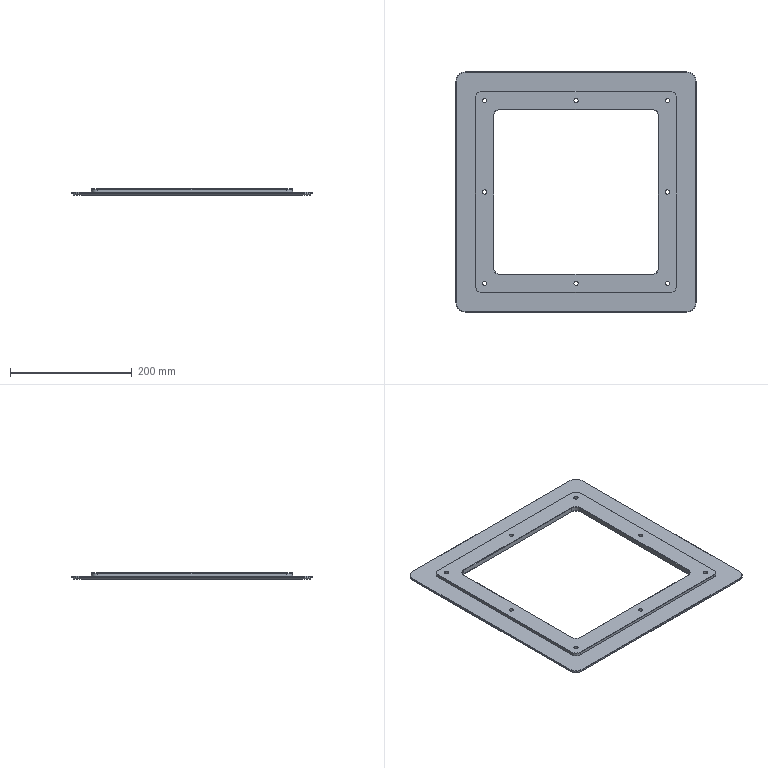NC program | Mastercam | posted with a generic post
Lines 2442 to 3195 of 5147:
N4630 T14 M6
N4640 G0 G90 G17 G54 X-208.453 Y181.943 A0. S1600 M3
N4650 G43 H14 Z50. M8
N4660 Z2.5
N4670 G1 Z1.22 F600.
N4680 G3 X-208.04 Y182.034 I-.234 J2.05 F3000.
N4690 X-207.654 Y182.207 I-.647 J1.959
N4700 X-207.312 Y182.455 I-1.033 J1.786
N4710 X-207.027 Y182.768 I-1.375 J1.538
N4720 G2 X-182.755 Y207.035 I92.551 J-68.297
N4730 G3 X-182.444 Y207.318 I-1.224 J1.66
N4740 X-182.197 Y207.657 I-1.535 J1.377
N4750 X-182.024 Y208.039 I-1.782 J1.038
N4760 X-181.932 Y208.449 I-1.955 J.656
N4770 G0 Z50.
N4780 X-208.443 Y151.131
N4790 Z2.5
N4800 G1 Z1.22 F600.
N4810 G3 X-207.997 Y151.303 I-.516 J1.997 F3000.
N4820 X-207.603 Y151.574 I-.962 J1.825
N4830 X-207.281 Y151.928 I-1.356 J1.554
N4840 X-207.05 Y152.347 I-1.678 J1.2
N4850 G2 X-156.896 Y205.053 I92.576 J-37.878
N4860 X-152.321 Y207.05 I42.587 J-91.317
N4870 G3 X-151.902 Y207.281 I-.778 J1.91
N4880 X-151.547 Y207.602 I-1.197 J1.679
N4890 X-151.276 Y207.996 I-1.552 J1.358
N4900 X-151.103 Y208.443 I-1.823 J.964
N4910 G0 Z50.
N4920 X181.945 Y208.453
N4930 Z2.5
N4940 G1 Z1.22 F600.
N4950 G3 X182.036 Y208.04 I2.05 J.234 F3000.
N4960 X182.209 Y207.654 I1.959 J.647
N4970 X182.457 Y207.312 I1.786 J1.033
N4980 X182.77 Y207.027 I1.538 J1.375
N4990 G2 X207.035 Y182.756 I-68.295 J-92.543
N5000 G3 X207.317 Y182.445 I1.66 J1.224
N5010 X207.657 Y182.198 I1.378 J1.535
N5020 X208.039 Y182.025 I1.038 J1.782
N5030 X208.449 Y181.932 I.656 J1.955
N5040 G0 Z50.
N5050 X151.134 Y208.443
N5060 Z2.5
N5070 G1 Z1.22 F600.
N5080 G3 X151.307 Y207.997 I1.997 J.516 F3000.
N5090 X151.577 Y207.603 I1.824 J.962
N5100 X151.931 Y207.281 I1.554 J1.356
N5110 X152.35 Y207.05 I1.2 J1.678
N5120 G2 X207.05 Y152.338 I-37.876 J-92.567
N5130 G3 X207.281 Y151.919 I1.909 J.78
N5140 X207.603 Y151.565 I1.678 J1.199
N5150 X207.997 Y151.294 I1.356 J1.553
N5160 X208.443 Y151.121 I.962 J1.824
N5170 G0 Z50.
N5180 X208.453 Y-181.945
N5190 Z2.5
N5200 G1 Z1.22 F600.
N5210 G3 X208.04 Y-182.036 I.234 J-2.05 F3000.
N5220 X207.654 Y-182.209 I.647 J-1.959
N5230 X207.312 Y-182.457 I1.033 J-1.786
N5240 X207.027 Y-182.77 I1.375 J-1.538
N5250 G2 X182.756 Y-207.035 I-92.543 J68.295
N5260 G3 X182.445 Y-207.317 I1.224 J-1.66
N5270 X182.198 Y-207.657 I1.535 J-1.378
N5280 X182.025 Y-208.039 I1.782 J-1.038
N5290 X181.932 Y-208.449 I1.955 J-.656
N5300 G0 Z50.
N5310 X208.443 Y-151.134
N5320 Z2.5
N5330 G1 Z1.22 F600.
N5340 G3 X207.997 Y-151.307 I.516 J-1.997 F3000.
N5350 X207.603 Y-151.577 I.962 J-1.824
N5360 X207.281 Y-151.931 I1.356 J-1.554
N5370 X207.05 Y-152.35 I1.678 J-1.2
N5380 G2 X152.338 Y-207.05 I-92.567 J37.876
N5390 G3 X151.919 Y-207.281 I.78 J-1.909
N5400 X151.565 Y-207.603 I1.199 J-1.678
N5410 X151.294 Y-207.997 I1.553 J-1.356
N5420 X151.121 Y-208.443 I1.824 J-.962
N5430 G0 Z50.
N5440 X-181.945 Y-208.453
N5450 Z2.5
N5460 G1 Z1.22 F600.
N5470 G3 X-182.036 Y-208.04 I-2.05 J-.234 F3000.
N5480 X-182.209 Y-207.654 I-1.959 J-.647
N5490 X-182.457 Y-207.312 I-1.786 J-1.033
N5500 X-182.77 Y-207.027 I-1.538 J-1.375
N5510 G2 X-207.032 Y-182.76 I68.295 J92.543
N5520 G3 X-207.315 Y-182.449 I-1.66 J-1.225
N5530 X-207.655 Y-182.202 I-1.377 J-1.536
N5540 X-208.038 Y-182.029 I-1.037 J-1.783
N5550 X-208.448 Y-181.937 I-.654 J-1.956
N5560 G0 Z50.
N5570 X-151.134 Y-208.443
N5580 Z2.5
N5590 G1 Z1.22 F600.
N5600 G3 X-151.307 Y-207.997 I-1.997 J-.516 F3000.
N5610 X-151.577 Y-207.603 I-1.824 J-.962
N5620 X-151.931 Y-207.281 I-1.554 J-1.356
N5630 X-152.35 Y-207.05 I-1.2 J-1.678
N5640 G2 X-207.05 Y-152.338 I37.876 J92.567
N5650 X-207.204 Y-151.557 I1.909 J.781
N5660 X-206.268 Y-149.83 I2.063 J0.
N5670 G1 X-196.136 Y-143.222
N5680 G3 X-195.2 Y-141.494 I-1.127 J1.728
N5690 X-195.302 Y-140.854 I-2.063 J0.
N5700 G2 X-196.868 Y-135.457 I80.827 J26.377
N5710 X-199.499 Y-114.308 I91.934 J22.176
N5720 G1 Y114.308
N5730 Y114.468
N5740 G2 X-150.463 Y191.502 I85.027 J0.
N5750 X-117.748 Y199.427 I36.203 J-77.967
N5760 G1 X0. Y199.499
N5770 X114.308
N5780 X114.475
N5790 G2 X196.868 Y135.457 I0. J-85.022
N5800 X199.499 Y114.308 I-91.934 J-22.176
N5810 G1 Y-114.308
N5820 Y-114.475
N5830 G2 X135.457 Y-196.868 I-85.022 J0.
N5840 X114.308 Y-199.499 I-22.176 J91.934
N5850 G1 X-114.308
N5860 X-114.475
N5870 G2 X-195.302 Y-140.854 I0. J85.022
N5880 X-195.404 Y-140.214 I1.961 J.64
N5890 X-194.347 Y-138.414 I2.063 J0.
N5900 G1 X-183.696 Y-132.466
N5910 G3 X-182.639 Y-130.665 I-1.005 J1.801
N5920 X-182.684 Y-130.238 I-2.062 J0.
N5930 G2 X-184.499 Y-114.308 I82.598 J17.483
N5940 G1 Y114.308
N5950 Y114.471
N5960 G2 X-138.139 Y180.374 I70.022 J0.
N5970 X-116.261 Y184.467 I24.165 J-68.647
N5980 G1 X0. Y184.499
N5990 X114.308
N6000 X114.475
N6010 G2 X182.506 Y131.058 I0. J-70.022
N6020 X184.499 Y114.308 I-82.42 J-18.303
N6030 G1 Y-114.308
N6040 Y-114.475
N6050 G2 X131.058 Y-182.506 I-70.022 J0.
N6060 X114.308 Y-184.499 I-18.303 J82.42
N6070 G1 X-114.308
N6080 X-114.475
N6090 G2 X-182.506 Y-131.058 I0. J70.022
N6100 X-182.684 Y-130.238 I82.42 J18.303
N6110 X-182.729 Y-129.811 I2.018 J.427
N6120 X-181.514 Y-127.931 I2.063 J0.
N6130 G1 X-170.282 Y-122.865
N6140 G3 X-169.068 Y-120.985 I-.848 J1.88
N6150 X-169.08 Y-120.76 I-2.062 J0.
N6160 G2 X-169.499 Y-114.308 I72.731 J7.973
N6170 G1 Y114.308
N6180 Y114.47
N6190 G2 X-132.181 Y166.568 I55.024 J0.
N6200 X-115.773 Y169.476 I18.581 J-57.102
N6210 G1 X0. Y169.499
N6220 X114.308
N6230 X114.473
N6240 G2 X168.498 Y124.943 I0. J-55.031
N6250 X169.499 Y114.308 I-72.149 J-12.156
N6260 G1 Y-114.308
N6270 Y-114.473
N6280 G2 X124.943 Y-168.498 I-55.031 J0.
N6290 X114.308 Y-169.499 I-12.156 J72.149
N6300 G1 X-114.308
N6310 X-114.473
N6320 G2 X-168.498 Y-124.943 I0. J55.031
N6330 X-169.08 Y-120.76 I72.149 J12.156
N6340 X-169.092 Y-120.535 I2.051 J.225
N6350 X-167.644 Y-118.567 I2.063 J0.
N6360 G1 X-155.947 Y-114.911
N6370 G3 X-154.5 Y-112.943 I-.615 J1.968
N6380 G1 Y114.308
N6390 Y114.469
N6400 G2 X-124.564 Y153.207 I40.032 J0.
N6410 X-114.308 Y154.5 I11.707 J-51.549
N6420 G1 X0.
N6430 X114.308
N6440 X114.479
N6450 G2 X154.078 Y120.224 I0. J-40.013
N6460 X154.5 Y114.308 I-47.356 J-6.345
N6470 G1 Y-114.308
N6480 Y-114.479
N6490 G2 X120.224 Y-154.078 I-40.013 J0.
N6500 X114.308 Y-154.5 I-6.345 J47.356
N6510 G1 X-114.308
N6520 X-114.479
N6530 G2 X-154.078 Y-120.224 I0. J40.013
N6540 X-154.5 Y-114.308 I47.356 J6.345
N6550 G1 Y-112.943
N6560 G2 X-152.809 Y-110.914 I2.063 J0.
N6570 G1 X-141.183 Y-108.783
N6580 G3 X-139.492 Y-106.755 I-.372 J2.028
N6590 G1 X-139.5 Y114.308
N6600 Y114.465
N6610 G2 X-119.184 Y139.057 I25.041 J0.
N6620 X-114.308 Y139.5 I5.273 J-30.972
N6630 G1 X0.
N6640 X114.308
N6650 G2 X114.476 Y139.501 I.168 J-25.018
N6660 X139.339 Y117.266 I0. J-25.019
N6670 G1 X139.492 Y114.796
N6680 X139.5 Y-114.308
N6690 G2 X139.501 Y-114.476 I-25.018 J-.168
N6700 X117.266 Y-139.339 I-25.019 J0.
N6710 G1 X114.796 Y-139.492
N6720 X-114.308 Y-139.5
N6730 G2 X-114.476 Y-139.501 I-.168 J25.018
N6740 X-139.339 Y-117.266 I0. J25.019
N6750 G1 X-139.492 Y-114.796
N6760 Y-106.755
N6770 G2 X-137.802 Y-104.726 I2.062 J0.
N6780 G1 X-126.19 Y-102.596
N6790 G3 X-124.5 Y-100.567 I-.373 J2.029
N6800 G1 Y114.308
N6810 G2 X-124.502 Y114.496 I10.002 J.188
N6820 X-115.306 Y124.467 I10.004 J0.
N6830 G1 X-114.308 Y124.5
N6840 X0.
N6850 X114.308
N6860 G2 X114.496 Y124.502 I.188 J-10.002
N6870 X124.467 Y115.306 I0. J-10.004
N6880 G1 X124.5 Y114.308
N6890 Y-114.308
N6900 G2 X124.502 Y-114.496 I-10.002 J-.188
N6910 X115.306 Y-124.467 I-10.004 J0.
N6920 G1 X114.308 Y-124.5
N6930 X-114.308
N6940 G2 X-114.496 Y-124.502 I-.188 J10.002
N6950 X-124.467 Y-115.306 I0. J10.004
N6960 G1 X-124.5 Y-114.308
N6970 Y-100.567
N6980 G0 Z50.
N6990 X-208.453 Y181.943
N7000 Z2.22
N7010 G1 Z.94 F600.
N7020 G3 X-208.04 Y182.034 I-.234 J2.05 F3000.
N7030 X-207.654 Y182.207 I-.647 J1.959
N7040 X-207.312 Y182.455 I-1.033 J1.786
N7050 X-207.027 Y182.768 I-1.375 J1.538
N7060 G2 X-182.755 Y207.035 I92.551 J-68.297
N7070 G3 X-182.444 Y207.318 I-1.224 J1.66
N7080 X-182.197 Y207.657 I-1.535 J1.377
N7090 X-182.024 Y208.039 I-1.782 J1.038
N7100 X-181.932 Y208.449 I-1.955 J.656
N7110 G0 Z50.
N7120 X-208.443 Y151.131
N7130 Z2.22
N7140 G1 Z.94 F600.
N7150 G3 X-207.997 Y151.303 I-.516 J1.997 F3000.
N7160 X-207.603 Y151.574 I-.962 J1.825
N7170 X-207.281 Y151.928 I-1.356 J1.554
N7180 X-207.05 Y152.347 I-1.678 J1.2
N7190 G2 X-156.896 Y205.053 I92.576 J-37.878
N7200 X-152.321 Y207.05 I42.587 J-91.317
N7210 G3 X-151.902 Y207.281 I-.778 J1.91
N7220 X-151.547 Y207.602 I-1.197 J1.679
N7230 X-151.276 Y207.996 I-1.552 J1.358
N7240 X-151.103 Y208.443 I-1.823 J.964
N7250 G0 Z50.
N7260 X181.945 Y208.453
N7270 Z2.22
N7280 G1 Z.94 F600.
N7290 G3 X182.036 Y208.04 I2.05 J.234 F3000.
N7300 X182.209 Y207.654 I1.959 J.647
N7310 X182.457 Y207.312 I1.786 J1.033
N7320 X182.77 Y207.027 I1.538 J1.375
N7330 G2 X207.035 Y182.756 I-68.295 J-92.543
N7340 G3 X207.317 Y182.445 I1.66 J1.224
N7350 X207.657 Y182.198 I1.378 J1.535
N7360 X208.039 Y182.025 I1.038 J1.782
N7370 X208.449 Y181.932 I.656 J1.955
N7380 G0 Z50.
N7390 X151.134 Y208.443
N7400 Z2.22
N7410 G1 Z.94 F600.
N7420 G3 X151.307 Y207.997 I1.997 J.516 F3000.
N7430 X151.577 Y207.603 I1.824 J.962
N7440 X151.931 Y207.281 I1.554 J1.356
N7450 X152.35 Y207.05 I1.2 J1.678
N7460 G2 X207.05 Y152.338 I-37.876 J-92.567
N7470 G3 X207.281 Y151.919 I1.909 J.78
N7480 X207.603 Y151.565 I1.678 J1.199
N7490 X207.997 Y151.294 I1.356 J1.553
N7500 X208.443 Y151.121 I.962 J1.824
N7510 G0 Z50.
N7520 X208.453 Y-181.945
N7530 Z2.22
N7540 G1 Z.94 F600.
N7550 G3 X208.04 Y-182.036 I.234 J-2.05 F3000.
N7560 X207.654 Y-182.209 I.647 J-1.959
N7570 X207.312 Y-182.457 I1.033 J-1.786
N7580 X207.027 Y-182.77 I1.375 J-1.538
N7590 G2 X182.756 Y-207.035 I-92.543 J68.295
N7600 G3 X182.445 Y-207.317 I1.224 J-1.66
N7610 X182.198 Y-207.657 I1.535 J-1.378
N7620 X182.025 Y-208.039 I1.782 J-1.038
N7630 X181.932 Y-208.449 I1.955 J-.656
N7640 G0 Z50.
N7650 X208.443 Y-151.134
N7660 Z2.22
N7670 G1 Z.94 F600.
N7680 G3 X207.997 Y-151.307 I.516 J-1.997 F3000.
N7690 X207.603 Y-151.577 I.962 J-1.824
N7700 X207.281 Y-151.931 I1.356 J-1.554
N7710 X207.05 Y-152.35 I1.678 J-1.2
N7720 G2 X152.338 Y-207.05 I-92.567 J37.876
N7730 G3 X151.919 Y-207.281 I.78 J-1.909
N7740 X151.565 Y-207.603 I1.199 J-1.678
N7750 X151.294 Y-207.997 I1.553 J-1.356
N7760 X151.121 Y-208.443 I1.824 J-.962
N7770 G0 Z50.
N7780 X-181.945 Y-208.453
N7790 Z2.22
N7800 G1 Z.94 F600.
N7810 G3 X-182.036 Y-208.04 I-2.05 J-.234 F3000.
N7820 X-182.209 Y-207.654 I-1.959 J-.647
N7830 X-182.457 Y-207.312 I-1.786 J-1.033
N7840 X-182.77 Y-207.027 I-1.538 J-1.375
N7850 G2 X-207.032 Y-182.76 I68.295 J92.543
N7860 G3 X-207.315 Y-182.449 I-1.66 J-1.225
N7870 X-207.655 Y-182.202 I-1.377 J-1.536
N7880 X-208.038 Y-182.029 I-1.037 J-1.783
N7890 X-208.448 Y-181.937 I-.654 J-1.956
N7900 G0 Z50.
N7910 X-151.134 Y-208.443
N7920 Z2.22
N7930 G1 Z.94 F600.
N7940 G3 X-151.307 Y-207.997 I-1.997 J-.516 F3000.
N7950 X-151.577 Y-207.603 I-1.824 J-.962
N7960 X-151.931 Y-207.281 I-1.554 J-1.356
N7970 X-152.35 Y-207.05 I-1.2 J-1.678
N7980 G2 X-207.05 Y-152.338 I37.876 J92.567
N7990 X-207.204 Y-151.557 I1.909 J.781
N8000 X-206.268 Y-149.83 I2.063 J0.
N8010 G1 X-196.136 Y-143.222
N8020 G3 X-195.2 Y-141.494 I-1.127 J1.728
N8030 X-195.302 Y-140.854 I-2.063 J0.
N8040 G2 X-196.868 Y-135.457 I80.827 J26.377
N8050 X-199.499 Y-114.308 I91.934 J22.176
N8060 G1 Y114.308
N8070 Y114.468
N8080 G2 X-150.463 Y191.502 I85.027 J0.
N8090 X-117.748 Y199.427 I36.203 J-77.967
N8100 G1 X0. Y199.499
N8110 X114.308
N8120 X114.475
N8130 G2 X196.868 Y135.457 I0. J-85.022
N8140 X199.499 Y114.308 I-91.934 J-22.176
N8150 G1 Y-114.308
N8160 Y-114.475
N8170 G2 X135.457 Y-196.868 I-85.022 J0.
N8180 X114.308 Y-199.499 I-22.176 J91.934
N8190 G1 X-114.308
N8200 X-114.475
N8210 G2 X-195.302 Y-140.854 I0. J85.022
N8220 X-195.404 Y-140.214 I1.961 J.64
N8230 X-194.347 Y-138.414 I2.063 J0.
N8240 G1 X-183.696 Y-132.466
N8250 G3 X-182.639 Y-130.665 I-1.005 J1.801
N8260 X-182.684 Y-130.238 I-2.062 J0.
N8270 G2 X-184.499 Y-114.308 I82.598 J17.483
N8280 G1 Y114.308
N8290 Y114.471
N8300 G2 X-138.139 Y180.374 I70.022 J0.
N8310 X-116.261 Y184.467 I24.165 J-68.647
N8320 G1 X0. Y184.499
N8330 X114.308
N8340 X114.475
N8350 G2 X182.506 Y131.058 I0. J-70.022
N8360 X184.499 Y114.308 I-82.42 J-18.303
N8370 G1 Y-114.308
N8380 Y-114.475
N8390 G2 X131.058 Y-182.506 I-70.022 J0.
N8400 X114.308 Y-184.499 I-18.303 J82.42
N8410 G1 X-114.308
N8420 X-114.475
N8430 G2 X-182.506 Y-131.058 I0. J70.022
N8440 X-182.684 Y-130.238 I82.42 J18.303
N8450 X-182.729 Y-129.811 I2.018 J.427
N8460 X-181.514 Y-127.931 I2.063 J0.
N8470 G1 X-170.282 Y-122.865
N8480 G3 X-169.068 Y-120.985 I-.848 J1.88
N8490 X-169.08 Y-120.76 I-2.062 J0.
N8500 G2 X-169.499 Y-114.308 I72.731 J7.973
N8510 G1 Y114.308
N8520 Y114.47
N8530 G2 X-132.181 Y166.568 I55.024 J0.
N8540 X-115.773 Y169.476 I18.581 J-57.102
N8550 G1 X0. Y169.499
N8560 X114.308
N8570 X114.473
N8580 G2 X168.498 Y124.943 I0. J-55.031
N8590 X169.499 Y114.308 I-72.149 J-12.156
N8600 G1 Y-114.308
N8610 Y-114.473
N8620 G2 X124.943 Y-168.498 I-55.031 J0.
N8630 X114.308 Y-169.499 I-12.156 J72.149
N8640 G1 X-114.308
N8650 X-114.473
N8660 G2 X-168.498 Y-124.943 I0. J55.031
N8670 X-169.08 Y-120.76 I72.149 J12.156
N8680 X-169.092 Y-120.535 I2.051 J.225
N8690 X-167.644 Y-118.567 I2.063 J0.
N8700 G1 X-155.947 Y-114.911
N8710 G3 X-154.5 Y-112.943 I-.615 J1.968
N8720 G1 Y114.308
N8730 Y114.469
N8740 G2 X-124.564 Y153.207 I40.032 J0.
N8750 X-114.308 Y154.5 I11.707 J-51.549
N8760 G1 X0.
N8770 X114.308
N8780 X114.479
N8790 G2 X154.078 Y120.224 I0. J-40.013
N8800 X154.5 Y114.308 I-47.356 J-6.345
N8810 G1 Y-114.308
N8820 Y-114.479
N8830 G2 X120.224 Y-154.078 I-40.013 J0.
N8840 X114.308 Y-154.5 I-6.345 J47.356
N8850 G1 X-114.308
N8860 X-114.479
N8870 G2 X-154.078 Y-120.224 I0. J40.013
N8880 X-154.5 Y-114.308 I47.356 J6.345
N8890 G1 Y-112.943
N8900 G2 X-152.809 Y-110.914 I2.063 J0.
N8910 G1 X-141.183 Y-108.783
N8920 G3 X-139.492 Y-106.755 I-.372 J2.028
N8930 G1 X-139.5 Y114.308
N8940 Y114.465
N8950 G2 X-119.184 Y139.057 I25.041 J0.
N8960 X-114.308 Y139.5 I5.273 J-30.972
N8970 G1 X0.
N8980 X114.308
N8990 G2 X114.476 Y139.501 I.168 J-25.018
N9000 X139.339 Y117.266 I0. J-25.019
N9010 G1 X139.492 Y114.796
N9020 X139.5 Y-114.308
N9030 G2 X139.501 Y-114.476 I-25.018 J-.168
N9040 X117.266 Y-139.339 I-25.019 J0.
N9050 G1 X114.796 Y-139.492
N9060 X-114.308 Y-139.5
N9070 G2 X-114.476 Y-139.501 I-.168 J25.018
N9080 X-139.339 Y-117.266 I0. J25.019
N9090 G1 X-139.492 Y-114.796
N9100 Y-106.755
N9110 G2 X-137.802 Y-104.726 I2.062 J0.
N9120 G1 X-126.19 Y-102.596
N9130 G3 X-124.5 Y-100.567 I-.373 J2.029
N9140 G1 Y114.308
N9150 G2 X-124.502 Y114.496 I10.002 J.188
N9160 X-115.306 Y124.467 I10.004 J0.
N9170 G1 X-114.308 Y124.5
N9180 X0.
N9190 X114.308
N9200 G2 X114.496 Y124.502 I.188 J-10.002
N9210 X124.467 Y115.306 I0. J-10.004
N9220 G1 X124.5 Y114.308
N9230 Y-114.308
N9240 G2 X124.502 Y-114.496 I-10.002 J-.188
N9250 X115.306 Y-124.467 I-10.004 J0.
N9260 G1 X114.308 Y-124.5
N9270 X-114.308
N9280 G2 X-114.496 Y-124.502 I-.188 J10.002
N9290 X-124.467 Y-115.306 I0. J10.004
N9300 G1 X-124.5 Y-114.308
N9310 Y-100.567
N9320 G0 Z50.
N9330 X-208.453 Y181.943
N9340 Z1.94
N9350 G1 Z.66 F600.
N9360 G3 X-208.04 Y182.034 I-.234 J2.05 F3000.
N9370 X-207.654 Y182.207 I-.647 J1.959
N9380 X-207.312 Y182.455 I-1.033 J1.786
N9390 X-207.027 Y182.768 I-1.375 J1.538
N9400 G2 X-182.755 Y207.035 I92.551 J-68.297
N9410 G3 X-182.444 Y207.318 I-1.224 J1.66
N9420 X-182.197 Y207.657 I-1.535 J1.377
N9430 X-182.024 Y208.039 I-1.782 J1.038
N9440 X-181.932 Y208.449 I-1.955 J.656
N9450 G0 Z50.
N9460 X-208.443 Y151.131
N9470 Z1.94
N9480 G1 Z.66 F600.
N9490 G3 X-207.997 Y151.303 I-.516 J1.997 F3000.
N9500 X-207.603 Y151.574 I-.962 J1.825
N9510 X-207.281 Y151.928 I-1.356 J1.554
N9520 X-207.05 Y152.347 I-1.678 J1.2
N9530 G2 X-156.896 Y205.053 I92.576 J-37.878
N9540 X-152.321 Y207.05 I42.587 J-91.317
N9550 G3 X-151.902 Y207.281 I-.778 J1.91
N9560 X-151.547 Y207.602 I-1.197 J1.679
N9570 X-151.276 Y207.996 I-1.552 J1.358
N9580 X-151.103 Y208.443 I-1.823 J.964
N9590 G0 Z50.
N9600 X181.945 Y208.453
N9610 Z1.94
N9620 G1 Z.66 F600.
N9630 G3 X182.036 Y208.04 I2.05 J.234 F3000.
N9640 X182.209 Y207.654 I1.959 J.647
N9650 X182.457 Y207.312 I1.786 J1.033
N9660 X182.77 Y207.027 I1.538 J1.375
N9670 G2 X207.035 Y182.756 I-68.295 J-92.543
N9680 G3 X207.317 Y182.445 I1.66 J1.224
N9690 X207.657 Y182.198 I1.378 J1.535
N9700 X208.039 Y182.025 I1.038 J1.782
N9710 X208.449 Y181.932 I.656 J1.955
N9720 G0 Z50.
N9730 X151.134 Y208.443
N9740 Z1.94
N9750 G1 Z.66 F600.
N9760 G3 X151.307 Y207.997 I1.997 J.516 F3000.
N9770 X151.577 Y207.603 I1.824 J.962
N9780 X151.931 Y207.281 I1.554 J1.356
N9790 X152.35 Y207.05 I1.2 J1.678
N9800 G2 X207.05 Y152.338 I-37.876 J-92.567
N9810 G3 X207.281 Y151.919 I1.909 J.78
N9820 X207.603 Y151.565 I1.678 J1.199
N9830 X207.997 Y151.294 I1.356 J1.553
N9840 X208.443 Y151.121 I.962 J1.824
N9850 G0 Z50.
N9860 X208.453 Y-181.945
N9870 Z1.94
N9880 G1 Z.66 F600.
N9890 G3 X208.04 Y-182.036 I.234 J-2.05 F3000.
N9900 X207.654 Y-182.209 I.647 J-1.959
N9910 X207.312 Y-182.457 I1.033 J-1.786
N9920 X207.027 Y-182.77 I1.375 J-1.538
N9930 G2 X182.756 Y-207.035 I-92.543 J68.295
N9940 G3 X182.445 Y-207.317 I1.224 J-1.66
N9950 X182.198 Y-207.657 I1.535 J-1.378
N9960 X182.025 Y-208.039 I1.782 J-1.038
N9970 X181.932 Y-208.449 I1.955 J-.656
N9980 G0 Z50.
N9990 X208.443 Y-151.134
N100 Z1.94
N110 G1 Z.66 F600.
N120 G3 X207.997 Y-151.307 I.516 J-1.997 F3000.
N130 X207.603 Y-151.577 I.962 J-1.824
N140 X207.281 Y-151.931 I1.356 J-1.554
N150 X207.05 Y-152.35 I1.678 J-1.2
N160 G2 X152.338 Y-207.05 I-92.567 J37.876
N170 G3 X151.919 Y-207.281 I.78 J-1.909
N180 X151.565 Y-207.603 I1.199 J-1.678
N190 X151.294 Y-207.997 I1.553 J-1.356
N200 X151.121 Y-208.443 I1.824 J-.962
N210 G0 Z50.
N220 X-181.945 Y-208.453
N230 Z1.94
N240 G1 Z.66 F600.
N250 G3 X-182.036 Y-208.04 I-2.05 J-.234 F3000.
N260 X-182.209 Y-207.654 I-1.959 J-.647
N270 X-182.457 Y-207.312 I-1.786 J-1.033
N280 X-182.77 Y-207.027 I-1.538 J-1.375
N290 G2 X-207.032 Y-182.76 I68.295 J92.543
N300 G3 X-207.315 Y-182.449 I-1.66 J-1.225
N310 X-207.655 Y-182.202 I-1.377 J-1.536
N320 X-208.038 Y-182.029 I-1.037 J-1.783
N330 X-208.448 Y-181.937 I-.654 J-1.956
N340 G0 Z50.
N350 X-151.134 Y-208.443
N360 Z1.94
N370 G1 Z.66 F600.
N380 G3 X-151.307 Y-207.997 I-1.997 J-.516 F3000.
N390 X-151.577 Y-207.603 I-1.824 J-.962
N400 X-151.931 Y-207.281 I-1.554 J-1.356
N410 X-152.35 Y-207.05 I-1.2 J-1.678
N420 G2 X-207.05 Y-152.338 I37.876 J92.567
N430 X-207.204 Y-151.557 I1.909 J.781
N440 X-206.268 Y-149.83 I2.063 J0.
N450 G1 X-196.136 Y-143.222
N460 G3 X-195.2 Y-141.494 I-1.127 J1.728
N470 X-195.302 Y-140.854 I-2.063 J0.
N480 G2 X-196.868 Y-135.457 I80.827 J26.377
N490 X-199.499 Y-114.308 I91.934 J22.176
N500 G1 Y114.308
N510 Y114.468
N520 G2 X-150.463 Y191.502 I85.027 J0.
N530 X-117.748 Y199.427 I36.203 J-77.967
N540 G1 X0. Y199.499
N550 X114.308
N560 X114.475
N570 G2 X196.868 Y135.457 I0. J-85.022
N580 X199.499 Y114.308 I-91.934 J-22.176
N590 G1 Y-114.308
N600 Y-114.475
N610 G2 X135.457 Y-196.868 I-85.022 J0.
N620 X114.308 Y-199.499 I-22.176 J91.934
N630 G1 X-114.308
N640 X-114.475
N650 G2 X-195.302 Y-140.854 I0. J85.022
N660 X-195.404 Y-140.214 I1.961 J.64
N670 X-194.347 Y-138.414 I2.063 J0.
N680 G1 X-183.696 Y-132.466
N690 G3 X-182.639 Y-130.665 I-1.005 J1.801
N700 X-182.684 Y-130.238 I-2.062 J0.
N710 G2 X-184.499 Y-114.308 I82.598 J17.483
N720 G1 Y114.308
N730 Y114.471
N740 G2 X-138.139 Y180.374 I70.022 J0.
N750 X-116.261 Y184.467 I24.165 J-68.647
N760 G1 X0. Y184.499
N770 X114.308
N780 X114.475
N790 G2 X182.506 Y131.058 I0. J-70.022
N800 X184.499 Y114.308 I-82.42 J-18.303
N810 G1 Y-114.308
N820 Y-114.475
N830 G2 X131.058 Y-182.506 I-70.022 J0.
N840 X114.308 Y-184.499 I-18.303 J82.42
N850 G1 X-114.308
N860 X-114.475
N870 G2 X-182.506 Y-131.058 I0. J70.022
N880 X-182.684 Y-130.238 I82.42 J18.303
N890 X-182.729 Y-129.811 I2.018 J.427
N900 X-181.514 Y-127.931 I2.063 J0.
N910 G1 X-170.282 Y-122.865
N920 G3 X-169.068 Y-120.985 I-.848 J1.88
N930 X-169.08 Y-120.76 I-2.062 J0.
N940 G2 X-169.499 Y-114.308 I72.731 J7.973
N950 G1 Y114.308
N960 Y114.47
N970 G2 X-132.181 Y166.568 I55.024 J0.
N980 X-115.773 Y169.476 I18.581 J-57.102
N990 G1 X0. Y169.499
N1000 X114.308
N1010 X114.473
N1020 G2 X168.498 Y124.943 I0. J-55.031
N1030 X169.499 Y114.308 I-72.149 J-12.156
N1040 G1 Y-114.308
N1050 Y-114.473
N1060 G2 X124.943 Y-168.498 I-55.031 J0.
N1070 X114.308 Y-169.499 I-12.156 J72.149
N1080 G1 X-114.308
N1090 X-114.473
N1100 G2 X-168.498 Y-124.943 I0. J55.031
N1110 X-169.08 Y-120.76 I72.149 J12.156
N1120 X-169.092 Y-120.535 I2.051 J.225
N1130 X-167.644 Y-118.567 I2.063 J0.
N1140 G1 X-155.947 Y-114.911
N1150 G3 X-154.5 Y-112.943 I-.615 J1.968
N1160 G1 Y114.308
N1170 Y114.469
N1180 G2 X-124.564 Y153.207 I40.032 J0.
N1190 X-114.308 Y154.5 I11.707 J-51.549
N1200 G1 X0.
N1210 X114.308
N1220 X114.479
N1230 G2 X154.078 Y120.224 I0. J-40.013
N1240 X154.5 Y114.308 I-47.356 J-6.345
N1250 G1 Y-114.308
N1260 Y-114.479
N1270 G2 X120.224 Y-154.078 I-40.013 J0.
N1280 X114.308 Y-154.5 I-6.345 J47.356
N1290 G1 X-114.308
N1300 X-114.479
N1310 G2 X-154.078 Y-120.224 I0. J40.013
N1320 X-154.5 Y-114.308 I47.356 J6.345
N1330 G1 Y-112.943
N1340 G2 X-152.809 Y-110.914 I2.063 J0.
N1350 G1 X-141.183 Y-108.783
N1360 G3 X-139.492 Y-106.755 I-.372 J2.028
N1370 G1 X-139.5 Y114.308
N1380 Y114.465
N1390 G2 X-119.184 Y139.057 I25.041 J0.
N1400 X-114.308 Y139.5 I5.273 J-30.972
N1410 G1 X0.
N1420 X114.308
N1430 G2 X114.476 Y139.501 I.168 J-25.018
N1440 X139.339 Y117.266 I0. J-25.019
N1450 G1 X139.492 Y114.796
N1460 X139.5 Y-114.308
N1470 G2 X139.501 Y-114.476 I-25.018 J-.168
N1480 X117.266 Y-139.339 I-25.019 J0.
N1490 G1 X114.796 Y-139.492
N1500 X-114.308 Y-139.5
N1510 G2 X-114.476 Y-139.501 I-.168 J25.018
N1520 X-139.339 Y-117.266 I0. J25.019
N1530 G1 X-139.492 Y-114.796
N1540 Y-106.755
N1550 G2 X-137.802 Y-104.726 I2.062 J0.
N1560 G1 X-126.19 Y-102.596
N1570 G3 X-124.5 Y-100.567 I-.373 J2.029
N1580 G1 Y114.308
N1590 G2 X-124.502 Y114.496 I10.002 J.188
N1600 X-115.306 Y124.467 I10.004 J0.
N1610 G1 X-114.308 Y124.5
N1620 X0.
N1630 X114.308
N1640 G2 X114.496 Y124.502 I.188 J-10.002
N1650 X124.467 Y115.306 I0. J-10.004
N1660 G1 X124.5 Y114.308
N1670 Y-114.308
N1680 G2 X124.502 Y-114.496 I-10.002 J-.188
N1690 X115.306 Y-124.467 I-10.004 J0.
N1700 G1 X114.308 Y-124.5
N1710 X-114.308
N1720 G2 X-114.496 Y-124.502 I-.188 J10.002
N1730 X-124.467 Y-115.306 I0. J10.004
N1740 G1 X-124.5 Y-114.308
N1750 Y-100.567
N1760 G0 Z50.
N1770 X-208.453 Y181.943
N1780 Z1.66
N1790 G1 Z.38 F600.
N1800 G3 X-208.04 Y182.034 I-.234 J2.05 F3000.
N1810 X-207.654 Y182.207 I-.647 J1.959
N1820 X-207.312 Y182.455 I-1.033 J1.786
N1830 X-207.027 Y182.768 I-1.375 J1.538
N1840 G2 X-182.755 Y207.035 I92.551 J-68.297
N1850 G3 X-182.444 Y207.318 I-1.224 J1.66
N1860 X-182.197 Y207.657 I-1.535 J1.377
N1870 X-182.024 Y208.039 I-1.782 J1.038
N1880 X-181.932 Y208.449 I-1.955 J.656
N1890 G0 Z50.
N1900 X-208.443 Y151.131
N1910 Z1.66
N1920 G1 Z.38 F600.
N1930 G3 X-207.997 Y151.303 I-.516 J1.997 F3000.
N1940 X-207.603 Y151.574 I-.962 J1.825
N1950 X-207.281 Y151.928 I-1.356 J1.554
N1960 X-207.05 Y152.347 I-1.678 J1.2
N1970 G2 X-156.896 Y205.053 I92.576 J-37.878
N1980 X-152.321 Y207.05 I42.587 J-91.317
N1990 G3 X-151.902 Y207.281 I-.778 J1.91
N2000 X-151.547 Y207.602 I-1.197 J1.679
N2010 X-151.276 Y207.996 I-1.552 J1.358
N2020 X-151.103 Y208.443 I-1.823 J.964
N2030 G0 Z50.
N2040 X181.945 Y208.453
N2050 Z1.66
N2060 G1 Z.38 F600.
N2070 G3 X182.036 Y208.04 I2.05 J.234 F3000.
N2080 X182.209 Y207.654 I1.959 J.647
N2090 X182.457 Y207.312 I1.786 J1.033
N2100 X182.77 Y207.027 I1.538 J1.375
N2110 G2 X207.035 Y182.756 I-68.295 J-92.543
N2120 G3 X207.317 Y182.445 I1.66 J1.224
N2130 X207.657 Y182.198 I1.378 J1.535
N2140 X208.039 Y182.025 I1.038 J1.782
N2150 X208.449 Y181.932 I.656 J1.955
N2160 G0 Z50.
N2170 X151.134 Y208.443
N2180 Z1.66
N2190 G1 Z.38 F600.
N2200 G3 X151.307 Y207.997 I1.997 J.516 F3000.
N2210 X151.577 Y207.603 I1.824 J.962
N2220 X151.931 Y207.281 I1.554 J1.356
N2230 X152.35 Y207.05 I1.2 J1.678
N2240 G2 X207.05 Y152.338 I-37.876 J-92.567
N2250 G3 X207.281 Y151.919 I1.909 J.78
N2260 X207.603 Y151.565 I1.678 J1.199